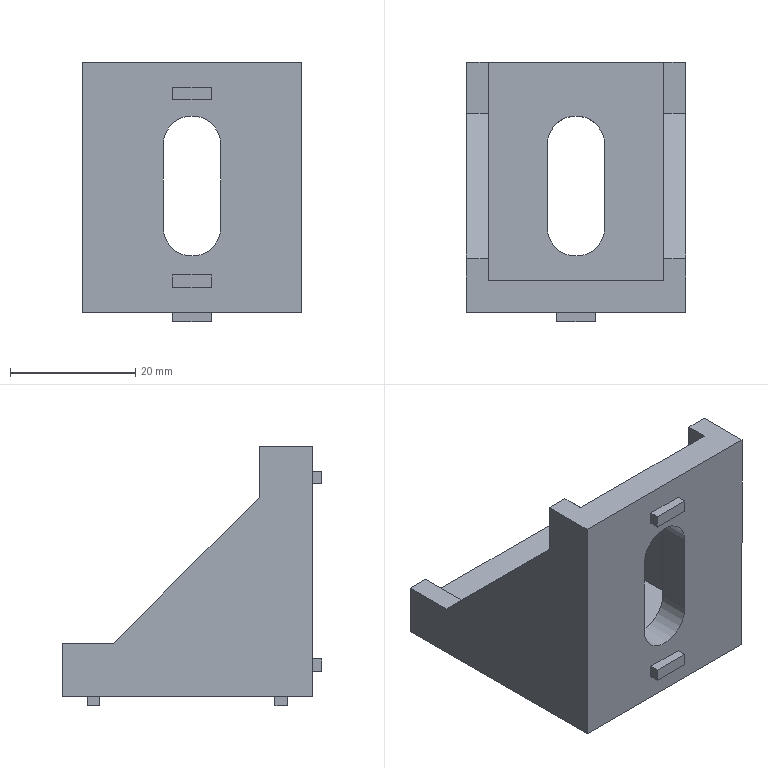Part | 1 solid | 44 faces | box 35 x 41.5 x 41.5 mm | volume 14850 mm3 | plane 40 | cylinder 4 | commonest cylinder face diameters 9.2 x4
STEP:
#1=CARTESIAN_POINT('',(14.,5.,5.));
#2=VERTEX_POINT('',#1);
#3=CARTESIAN_POINT('',(-14.,5.,5.));
#4=VERTEX_POINT('',#3);
#5=CARTESIAN_POINT('',(-17.5,5.,5.));
#6=DIRECTION('',(-1.,0.,0.));
#7=VECTOR('',#6,1000.);
#8=LINE('',#5,#7);
#9=EDGE_CURVE('',#2,#4,#8,.T.);
#10=ORIENTED_EDGE('',*,*,#9,.F.);
#11=CARTESIAN_POINT('',(14.,40.,5.));
#12=VERTEX_POINT('',#11);
#13=CARTESIAN_POINT('',(14.,0.,5.));
#14=DIRECTION('',(0.,-1.,0.));
#15=VECTOR('',#14,1000.);
#16=LINE('',#13,#15);
#17=EDGE_CURVE('',#12,#2,#16,.T.);
#18=ORIENTED_EDGE('',*,*,#17,.F.);
#19=CARTESIAN_POINT('',(-14.,40.,5.));
#20=VERTEX_POINT('',#19);
#21=CARTESIAN_POINT('',(-17.5,40.,5.));
#22=DIRECTION('',(-1.,0.,0.));
#23=VECTOR('',#22,1000.);
#24=LINE('',#21,#23);
#25=EDGE_CURVE('',#12,#20,#24,.T.);
#26=ORIENTED_EDGE('',*,*,#25,.T.);
#27=CARTESIAN_POINT('',(-14.,0.,5.));
#28=DIRECTION('',(0.,-1.,0.));
#29=VECTOR('',#28,1000.);
#30=LINE('',#27,#29);
#31=EDGE_CURVE('',#20,#4,#30,.T.);
#32=ORIENTED_EDGE('',*,*,#31,.T.);
#33=EDGE_LOOP('',(#10,#18,#26,#32));
#34=FACE_OUTER_BOUND('',#33,.T.);
#35=CARTESIAN_POINT('',(-4.6,26.8,5.));
#36=VERTEX_POINT('',#35);
#37=CARTESIAN_POINT('',(-4.6,13.6,5.));
#38=VERTEX_POINT('',#37);
#39=CARTESIAN_POINT('',(-4.6,26.8,5.));
#40=DIRECTION('',(0.,-1.,0.));
#41=VECTOR('',#40,1000.);
#42=LINE('',#39,#41);
#43=EDGE_CURVE('',#36,#38,#42,.T.);
#44=ORIENTED_EDGE('',*,*,#43,.F.);
#45=CARTESIAN_POINT('',(4.6,26.8,5.));
#46=VERTEX_POINT('',#45);
#47=CARTESIAN_POINT('',(0.,26.8,5.));
#48=DIRECTION('',(0.,0.,1.));
#49=DIRECTION('',(1.,0.,0.));
#50=AXIS2_PLACEMENT_3D('',#47,#48,#49);
#51=CIRCLE('',#50,4.6);
#52=EDGE_CURVE('',#46,#36,#51,.T.);
#53=ORIENTED_EDGE('',*,*,#52,.F.);
#54=CARTESIAN_POINT('',(4.6,13.6,5.));
#55=VERTEX_POINT('',#54);
#56=CARTESIAN_POINT('',(4.6,26.8,5.));
#57=DIRECTION('',(0.,1.,0.));
#58=VECTOR('',#57,1000.);
#59=LINE('',#56,#58);
#60=EDGE_CURVE('',#55,#46,#59,.T.);
#61=ORIENTED_EDGE('',*,*,#60,.F.);
#62=CARTESIAN_POINT('',(0.,13.6,5.));
#63=DIRECTION('',(0.,0.,1.));
#64=DIRECTION('',(1.,0.,0.));
#65=AXIS2_PLACEMENT_3D('',#62,#63,#64);
#66=CIRCLE('',#65,4.6);
#67=EDGE_CURVE('',#38,#55,#66,.T.);
#68=ORIENTED_EDGE('',*,*,#67,.F.);
#69=EDGE_LOOP('',(#44,#53,#61,#68));
#70=FACE_BOUND('',#69,.T.);
#71=CARTESIAN_POINT('',(-17.5,0.,5.));
#72=DIRECTION('',(0.,0.,1.));
#73=DIRECTION('',(1.,0.,0.));
#74=AXIS2_PLACEMENT_3D('',#71,#72,#73);
#75=PLANE('',#74);
#76=ADVANCED_FACE('',(#34,#70),#75,.T.);
#77=CARTESIAN_POINT('',(17.5,40.,0.));
#78=VERTEX_POINT('',#77);
#79=CARTESIAN_POINT('',(-17.5,40.,0.));
#80=VERTEX_POINT('',#79);
#81=CARTESIAN_POINT('',(-17.5,40.,0.));
#82=DIRECTION('',(-1.,0.,0.));
#83=VECTOR('',#82,1000.);
#84=LINE('',#81,#83);
#85=EDGE_CURVE('',#78,#80,#84,.T.);
#86=ORIENTED_EDGE('',*,*,#85,.F.);
#87=CARTESIAN_POINT('',(17.5,0.,0.));
#88=VERTEX_POINT('',#87);
#89=CARTESIAN_POINT('',(17.5,40.,0.));
#90=DIRECTION('',(0.,1.,0.));
#91=VECTOR('',#90,1000.);
#92=LINE('',#89,#91);
#93=EDGE_CURVE('',#88,#78,#92,.T.);
#94=ORIENTED_EDGE('',*,*,#93,.F.);
#95=CARTESIAN_POINT('',(-17.5,0.,0.));
#96=VERTEX_POINT('',#95);
#97=CARTESIAN_POINT('',(-17.5,0.,0.));
#98=DIRECTION('',(1.,0.,0.));
#99=VECTOR('',#98,1000.);
#100=LINE('',#97,#99);
#101=EDGE_CURVE('',#96,#88,#100,.T.);
#102=ORIENTED_EDGE('',*,*,#101,.F.);
#103=CARTESIAN_POINT('',(-17.5,40.,0.));
#104=DIRECTION('',(0.,-1.,0.));
#105=VECTOR('',#104,1000.);
#106=LINE('',#103,#105);
#107=EDGE_CURVE('',#80,#96,#106,.T.);
#108=ORIENTED_EDGE('',*,*,#107,.F.);
#109=EDGE_LOOP('',(#86,#94,#102,#108));
#110=FACE_OUTER_BOUND('',#109,.T.);
#111=CARTESIAN_POINT('',(3.1,34.,0.));
#112=VERTEX_POINT('',#111);
#113=CARTESIAN_POINT('',(-3.1,34.,0.));
#114=VERTEX_POINT('',#113);
#115=CARTESIAN_POINT('',(3.1,34.,0.));
#116=DIRECTION('',(-1.,0.,0.));
#117=VECTOR('',#116,1000.);
#118=LINE('',#115,#117);
#119=EDGE_CURVE('',#112,#114,#118,.T.);
#120=ORIENTED_EDGE('',*,*,#119,.F.);
#121=CARTESIAN_POINT('',(3.1,36.,0.));
#122=VERTEX_POINT('',#121);
#123=CARTESIAN_POINT('',(3.1,36.,0.));
#124=DIRECTION('',(0.,-1.,0.));
#125=VECTOR('',#124,1000.);
#126=LINE('',#123,#125);
#127=EDGE_CURVE('',#122,#112,#126,.T.);
#128=ORIENTED_EDGE('',*,*,#127,.F.);
#129=CARTESIAN_POINT('',(-3.1,36.,0.));
#130=VERTEX_POINT('',#129);
#131=CARTESIAN_POINT('',(3.1,36.,0.));
#132=DIRECTION('',(-1.,0.,0.));
#133=VECTOR('',#132,1000.);
#134=LINE('',#131,#133);
#135=EDGE_CURVE('',#122,#130,#134,.T.);
#136=ORIENTED_EDGE('',*,*,#135,.T.);
#137=CARTESIAN_POINT('',(-3.1,36.,0.));
#138=DIRECTION('',(0.,-1.,0.));
#139=VECTOR('',#138,1000.);
#140=LINE('',#137,#139);
#141=EDGE_CURVE('',#130,#114,#140,.T.);
#142=ORIENTED_EDGE('',*,*,#141,.T.);
#143=EDGE_LOOP('',(#120,#128,#136,#142));
#144=FACE_BOUND('',#143,.T.);
#145=CARTESIAN_POINT('',(3.1,4.,0.));
#146=VERTEX_POINT('',#145);
#147=CARTESIAN_POINT('',(-3.1,4.,0.));
#148=VERTEX_POINT('',#147);
#149=CARTESIAN_POINT('',(3.1,4.,0.));
#150=DIRECTION('',(-1.,0.,0.));
#151=VECTOR('',#150,1000.);
#152=LINE('',#149,#151);
#153=EDGE_CURVE('',#146,#148,#152,.T.);
#154=ORIENTED_EDGE('',*,*,#153,.F.);
#155=CARTESIAN_POINT('',(3.1,6.,0.));
#156=VERTEX_POINT('',#155);
#157=CARTESIAN_POINT('',(3.1,4.,0.));
#158=DIRECTION('',(0.,-1.,0.));
#159=VECTOR('',#158,1000.);
#160=LINE('',#157,#159);
#161=EDGE_CURVE('',#156,#146,#160,.T.);
#162=ORIENTED_EDGE('',*,*,#161,.F.);
#163=CARTESIAN_POINT('',(-3.1,6.,0.));
#164=VERTEX_POINT('',#163);
#165=CARTESIAN_POINT('',(3.1,6.,0.));
#166=DIRECTION('',(-1.,0.,0.));
#167=VECTOR('',#166,1000.);
#168=LINE('',#165,#167);
#169=EDGE_CURVE('',#156,#164,#168,.T.);
#170=ORIENTED_EDGE('',*,*,#169,.T.);
#171=CARTESIAN_POINT('',(-3.1,4.,0.));
#172=DIRECTION('',(0.,-1.,0.));
#173=VECTOR('',#172,1000.);
#174=LINE('',#171,#173);
#175=EDGE_CURVE('',#164,#148,#174,.T.);
#176=ORIENTED_EDGE('',*,*,#175,.T.);
#177=EDGE_LOOP('',(#154,#162,#170,#176));
#178=FACE_BOUND('',#177,.T.);
#179=CARTESIAN_POINT('',(4.6,26.8,0.));
#180=VERTEX_POINT('',#179);
#181=CARTESIAN_POINT('',(-4.6,26.8,0.));
#182=VERTEX_POINT('',#181);
#183=CARTESIAN_POINT('',(0.,26.8,0.));
#184=DIRECTION('',(0.,0.,1.));
#185=DIRECTION('',(1.,0.,0.));
#186=AXIS2_PLACEMENT_3D('',#183,#184,#185);
#187=CIRCLE('',#186,4.6);
#188=EDGE_CURVE('',#180,#182,#187,.T.);
#189=ORIENTED_EDGE('',*,*,#188,.T.);
#190=CARTESIAN_POINT('',(-4.6,13.6,0.));
#191=VERTEX_POINT('',#190);
#192=CARTESIAN_POINT('',(-4.6,26.8,0.));
#193=DIRECTION('',(0.,-1.,0.));
#194=VECTOR('',#193,1000.);
#195=LINE('',#192,#194);
#196=EDGE_CURVE('',#182,#191,#195,.T.);
#197=ORIENTED_EDGE('',*,*,#196,.T.);
#198=CARTESIAN_POINT('',(4.6,13.6,0.));
#199=VERTEX_POINT('',#198);
#200=CARTESIAN_POINT('',(0.,13.6,0.));
#201=DIRECTION('',(0.,0.,1.));
#202=DIRECTION('',(1.,0.,0.));
#203=AXIS2_PLACEMENT_3D('',#200,#201,#202);
#204=CIRCLE('',#203,4.6);
#205=EDGE_CURVE('',#191,#199,#204,.T.);
#206=ORIENTED_EDGE('',*,*,#205,.T.);
#207=CARTESIAN_POINT('',(4.6,26.8,0.));
#208=DIRECTION('',(0.,1.,0.));
#209=VECTOR('',#208,1000.);
#210=LINE('',#207,#209);
#211=EDGE_CURVE('',#199,#180,#210,.T.);
#212=ORIENTED_EDGE('',*,*,#211,.T.);
#213=EDGE_LOOP('',(#189,#197,#206,#212));
#214=FACE_BOUND('',#213,.T.);
#215=CARTESIAN_POINT('',(-17.5,0.,0.));
#216=DIRECTION('',(0.,0.,1.));
#217=DIRECTION('',(1.,0.,0.));
#218=AXIS2_PLACEMENT_3D('',#215,#216,#217);
#219=PLANE('',#218);
#220=ADVANCED_FACE('',(#110,#144,#178,#214),#219,.F.);
#221=ORIENTED_EDGE('',*,*,#107,.T.);
#222=CARTESIAN_POINT('',(-17.5,0.,40.));
#223=VERTEX_POINT('',#222);
#224=CARTESIAN_POINT('',(-17.5,0.,5.));
#225=DIRECTION('',(0.,0.,-1.));
#226=VECTOR('',#225,1000.);
#227=LINE('',#224,#226);
#228=EDGE_CURVE('',#223,#96,#227,.T.);
#229=ORIENTED_EDGE('',*,*,#228,.F.);
#230=CARTESIAN_POINT('',(-17.5,8.5,40.));
#231=VERTEX_POINT('',#230);
#232=CARTESIAN_POINT('',(-17.5,8.5,40.));
#233=DIRECTION('',(0.,1.,0.));
#234=VECTOR('',#233,1000.);
#235=LINE('',#232,#234);
#236=EDGE_CURVE('',#223,#231,#235,.T.);
#237=ORIENTED_EDGE('',*,*,#236,.T.);
#238=CARTESIAN_POINT('',(-17.5,8.5,31.8));
#239=VERTEX_POINT('',#238);
#240=CARTESIAN_POINT('',(-17.5,8.5,31.8));
#241=DIRECTION('',(0.,0.,-1.));
#242=VECTOR('',#241,1000.);
#243=LINE('',#240,#242);
#244=EDGE_CURVE('',#231,#239,#243,.T.);
#245=ORIENTED_EDGE('',*,*,#244,.T.);
#246=CARTESIAN_POINT('',(-17.5,31.8,8.5));
#247=VERTEX_POINT('',#246);
#248=CARTESIAN_POINT('',(-17.5,31.8,8.5));
#249=DIRECTION('',(0.,0.7071,-0.7071));
#250=VECTOR('',#249,1000.);
#251=LINE('',#248,#250);
#252=EDGE_CURVE('',#239,#247,#251,.T.);
#253=ORIENTED_EDGE('',*,*,#252,.T.);
#254=CARTESIAN_POINT('',(-17.5,40.,8.5));
#255=VERTEX_POINT('',#254);
#256=CARTESIAN_POINT('',(-17.5,40.,8.5));
#257=DIRECTION('',(0.,1.,0.));
#258=VECTOR('',#257,1000.);
#259=LINE('',#256,#258);
#260=EDGE_CURVE('',#247,#255,#259,.T.);
#261=ORIENTED_EDGE('',*,*,#260,.T.);
#262=CARTESIAN_POINT('',(-17.5,40.,5.));
#263=DIRECTION('',(0.,0.,-1.));
#264=VECTOR('',#263,1000.);
#265=LINE('',#262,#264);
#266=EDGE_CURVE('',#255,#80,#265,.T.);
#267=ORIENTED_EDGE('',*,*,#266,.T.);
#268=EDGE_LOOP('',(#221,#229,#237,#245,#253,#261,#267));
#269=FACE_OUTER_BOUND('',#268,.T.);
#270=CARTESIAN_POINT('',(-17.5,40.,5.));
#271=DIRECTION('',(1.,0.,0.));
#272=DIRECTION('',(0.,1.,0.));
#273=AXIS2_PLACEMENT_3D('',#270,#271,#272);
#274=PLANE('',#273);
#275=ADVANCED_FACE('',(#269),#274,.F.);
#276=CARTESIAN_POINT('',(17.5,0.,40.));
#277=VERTEX_POINT('',#276);
#278=CARTESIAN_POINT('',(17.5,0.,5.));
#279=DIRECTION('',(0.,0.,-1.));
#280=VECTOR('',#279,1000.);
#281=LINE('',#278,#280);
#282=EDGE_CURVE('',#277,#88,#281,.T.);
#283=ORIENTED_EDGE('',*,*,#282,.F.);
#284=CARTESIAN_POINT('',(-14.,0.,40.));
#285=DIRECTION('',(-1.,0.,0.));
#286=VECTOR('',#285,1000.);
#287=LINE('',#284,#286);
#288=EDGE_CURVE('',#277,#223,#287,.T.);
#289=ORIENTED_EDGE('',*,*,#288,.T.);
#290=ORIENTED_EDGE('',*,*,#228,.T.);
#291=ORIENTED_EDGE('',*,*,#101,.T.);
#292=EDGE_LOOP('',(#283,#289,#290,#291));
#293=FACE_OUTER_BOUND('',#292,.T.);
#294=CARTESIAN_POINT('',(3.1,0.,6.));
#295=VERTEX_POINT('',#294);
#296=CARTESIAN_POINT('',(-3.1,0.,6.));
#297=VERTEX_POINT('',#296);
#298=CARTESIAN_POINT('',(3.1,0.,6.));
#299=DIRECTION('',(-1.,0.,0.));
#300=VECTOR('',#299,1000.);
#301=LINE('',#298,#300);
#302=EDGE_CURVE('',#295,#297,#301,.T.);
#303=ORIENTED_EDGE('',*,*,#302,.F.);
#304=CARTESIAN_POINT('',(3.1,0.,4.));
#305=VERTEX_POINT('',#304);
#306=CARTESIAN_POINT('',(3.1,0.,4.));
#307=DIRECTION('',(0.,0.,1.));
#308=VECTOR('',#307,1000.);
#309=LINE('',#306,#308);
#310=EDGE_CURVE('',#305,#295,#309,.T.);
#311=ORIENTED_EDGE('',*,*,#310,.F.);
#312=CARTESIAN_POINT('',(-3.1,0.,4.));
#313=VERTEX_POINT('',#312);
#314=CARTESIAN_POINT('',(3.1,0.,4.));
#315=DIRECTION('',(-1.,0.,0.));
#316=VECTOR('',#315,1000.);
#317=LINE('',#314,#316);
#318=EDGE_CURVE('',#305,#313,#317,.T.);
#319=ORIENTED_EDGE('',*,*,#318,.T.);
#320=CARTESIAN_POINT('',(-3.1,0.,4.));
#321=DIRECTION('',(0.,0.,1.));
#322=VECTOR('',#321,1000.);
#323=LINE('',#320,#322);
#324=EDGE_CURVE('',#313,#297,#323,.T.);
#325=ORIENTED_EDGE('',*,*,#324,.T.);
#326=EDGE_LOOP('',(#303,#311,#319,#325));
#327=FACE_BOUND('',#326,.T.);
#328=CARTESIAN_POINT('',(3.1,0.,36.));
#329=VERTEX_POINT('',#328);
#330=CARTESIAN_POINT('',(-3.1,0.,36.));
#331=VERTEX_POINT('',#330);
#332=CARTESIAN_POINT('',(3.1,0.,36.));
#333=DIRECTION('',(-1.,0.,0.));
#334=VECTOR('',#333,1000.);
#335=LINE('',#332,#334);
#336=EDGE_CURVE('',#329,#331,#335,.T.);
#337=ORIENTED_EDGE('',*,*,#336,.F.);
#338=CARTESIAN_POINT('',(3.1,0.,34.));
#339=VERTEX_POINT('',#338);
#340=CARTESIAN_POINT('',(3.1,0.,36.));
#341=DIRECTION('',(0.,0.,1.));
#342=VECTOR('',#341,1000.);
#343=LINE('',#340,#342);
#344=EDGE_CURVE('',#339,#329,#343,.T.);
#345=ORIENTED_EDGE('',*,*,#344,.F.);
#346=CARTESIAN_POINT('',(-3.1,0.,34.));
#347=VERTEX_POINT('',#346);
#348=CARTESIAN_POINT('',(3.1,0.,34.));
#349=DIRECTION('',(-1.,0.,0.));
#350=VECTOR('',#349,1000.);
#351=LINE('',#348,#350);
#352=EDGE_CURVE('',#339,#347,#351,.T.);
#353=ORIENTED_EDGE('',*,*,#352,.T.);
#354=CARTESIAN_POINT('',(-3.1,0.,36.));
#355=DIRECTION('',(0.,0.,1.));
#356=VECTOR('',#355,1000.);
#357=LINE('',#354,#356);
#358=EDGE_CURVE('',#347,#331,#357,.T.);
#359=ORIENTED_EDGE('',*,*,#358,.T.);
#360=EDGE_LOOP('',(#337,#345,#353,#359));
#361=FACE_BOUND('',#360,.T.);
#362=CARTESIAN_POINT('',(-4.6,0.,26.8));
#363=VERTEX_POINT('',#362);
#364=CARTESIAN_POINT('',(-4.6,0.,13.6));
#365=VERTEX_POINT('',#364);
#366=CARTESIAN_POINT('',(-4.6,0.,26.8));
#367=DIRECTION('',(0.,0.,-1.));
#368=VECTOR('',#367,1000.);
#369=LINE('',#366,#368);
#370=EDGE_CURVE('',#363,#365,#369,.T.);
#371=ORIENTED_EDGE('',*,*,#370,.F.);
#372=CARTESIAN_POINT('',(4.6,0.,26.8));
#373=VERTEX_POINT('',#372);
#374=CARTESIAN_POINT('',(0.,0.,26.8));
#375=DIRECTION('',(0.,-1.,0.));
#376=DIRECTION('',(1.,0.,0.));
#377=AXIS2_PLACEMENT_3D('',#374,#375,#376);
#378=CIRCLE('',#377,4.6);
#379=EDGE_CURVE('',#373,#363,#378,.T.);
#380=ORIENTED_EDGE('',*,*,#379,.F.);
#381=CARTESIAN_POINT('',(4.6,0.,13.6));
#382=VERTEX_POINT('',#381);
#383=CARTESIAN_POINT('',(4.6,0.,26.8));
#384=DIRECTION('',(0.,0.,1.));
#385=VECTOR('',#384,1000.);
#386=LINE('',#383,#385);
#387=EDGE_CURVE('',#382,#373,#386,.T.);
#388=ORIENTED_EDGE('',*,*,#387,.F.);
#389=CARTESIAN_POINT('',(0.,0.,13.6));
#390=DIRECTION('',(0.,-1.,0.));
#391=DIRECTION('',(1.,0.,0.));
#392=AXIS2_PLACEMENT_3D('',#389,#390,#391);
#393=CIRCLE('',#392,4.6);
#394=EDGE_CURVE('',#365,#382,#393,.T.);
#395=ORIENTED_EDGE('',*,*,#394,.F.);
#396=EDGE_LOOP('',(#371,#380,#388,#395));
#397=FACE_BOUND('',#396,.T.);
#398=CARTESIAN_POINT('',(-17.5,0.,5.));
#399=DIRECTION('',(0.,1.,0.));
#400=DIRECTION('',(1.,0.,0.));
#401=AXIS2_PLACEMENT_3D('',#398,#399,#400);
#402=PLANE('',#401);
#403=ADVANCED_FACE('',(#293,#327,#361,#397),#402,.F.);
#404=CARTESIAN_POINT('',(17.5,8.5,40.));
#405=VERTEX_POINT('',#404);
#406=CARTESIAN_POINT('',(17.5,8.5,31.8));
#407=VERTEX_POINT('',#406);
#408=CARTESIAN_POINT('',(17.5,8.5,31.8));
#409=DIRECTION('',(0.,0.,-1.));
#410=VECTOR('',#409,1000.);
#411=LINE('',#408,#410);
#412=EDGE_CURVE('',#405,#407,#411,.T.);
#413=ORIENTED_EDGE('',*,*,#412,.F.);
#414=CARTESIAN_POINT('',(17.5,8.5,40.));
#415=DIRECTION('',(0.,1.,0.));
#416=VECTOR('',#415,1000.);
#417=LINE('',#414,#416);
#418=EDGE_CURVE('',#277,#405,#417,.T.);
#419=ORIENTED_EDGE('',*,*,#418,.F.);
#420=ORIENTED_EDGE('',*,*,#282,.T.);
#421=ORIENTED_EDGE('',*,*,#93,.T.);
#422=CARTESIAN_POINT('',(17.5,40.,8.5));
#423=VERTEX_POINT('',#422);
#424=CARTESIAN_POINT('',(17.5,40.,5.));
#425=DIRECTION('',(0.,0.,-1.));
#426=VECTOR('',#425,1000.);
#427=LINE('',#424,#426);
#428=EDGE_CURVE('',#423,#78,#427,.T.);
#429=ORIENTED_EDGE('',*,*,#428,.F.);
#430=CARTESIAN_POINT('',(17.5,31.8,8.5));
#431=VERTEX_POINT('',#430);
#432=CARTESIAN_POINT('',(17.5,40.,8.5));
#433=DIRECTION('',(0.,1.,0.));
#434=VECTOR('',#433,1000.);
#435=LINE('',#432,#434);
#436=EDGE_CURVE('',#431,#423,#435,.T.);
#437=ORIENTED_EDGE('',*,*,#436,.F.);
#438=CARTESIAN_POINT('',(17.5,31.8,8.5));
#439=DIRECTION('',(0.,0.7071,-0.7071));
#440=VECTOR('',#439,1000.);
#441=LINE('',#438,#440);
#442=EDGE_CURVE('',#407,#431,#441,.T.);
#443=ORIENTED_EDGE('',*,*,#442,.F.);
#444=EDGE_LOOP('',(#413,#419,#420,#421,#429,#437,#443));
#445=FACE_OUTER_BOUND('',#444,.T.);
#446=CARTESIAN_POINT('',(17.5,40.,5.));
#447=DIRECTION('',(-1.,0.,0.));
#448=DIRECTION('',(0.,1.,0.));
#449=AXIS2_PLACEMENT_3D('',#446,#447,#448);
#450=PLANE('',#449);
#451=ADVANCED_FACE('',(#445),#450,.F.);
#452=ORIENTED_EDGE('',*,*,#85,.T.);
#453=ORIENTED_EDGE('',*,*,#266,.F.);
#454=CARTESIAN_POINT('',(-14.,40.,8.5));
#455=VERTEX_POINT('',#454);
#456=CARTESIAN_POINT('',(-14.,40.,8.5));
#457=DIRECTION('',(-1.,0.,0.));
#458=VECTOR('',#457,1000.);
#459=LINE('',#456,#458);
#460=EDGE_CURVE('',#455,#255,#459,.T.);
#461=ORIENTED_EDGE('',*,*,#460,.F.);
#462=CARTESIAN_POINT('',(-14.,40.,5.));
#463=DIRECTION('',(0.,0.,-1.));
#464=VECTOR('',#463,1000.);
#465=LINE('',#462,#464);
#466=EDGE_CURVE('',#455,#20,#465,.T.);
#467=ORIENTED_EDGE('',*,*,#466,.T.);
#468=ORIENTED_EDGE('',*,*,#25,.F.);
#469=CARTESIAN_POINT('',(14.,40.,8.5));
#470=VERTEX_POINT('',#469);
#471=CARTESIAN_POINT('',(14.,40.,5.));
#472=DIRECTION('',(0.,0.,-1.));
#473=VECTOR('',#472,1000.);
#474=LINE('',#471,#473);
#475=EDGE_CURVE('',#470,#12,#474,.T.);
#476=ORIENTED_EDGE('',*,*,#475,.F.);
#477=CARTESIAN_POINT('',(14.,40.,8.5));
#478=DIRECTION('',(1.,0.,0.));
#479=VECTOR('',#478,1000.);
#480=LINE('',#477,#479);
#481=EDGE_CURVE('',#470,#423,#480,.T.);
#482=ORIENTED_EDGE('',*,*,#481,.T.);
#483=ORIENTED_EDGE('',*,*,#428,.T.);
#484=EDGE_LOOP('',(#452,#453,#461,#467,#468,#476,#482,#483));
#485=FACE_OUTER_BOUND('',#484,.T.);
#486=CARTESIAN_POINT('',(-17.5,40.,5.));
#487=DIRECTION('',(0.,-1.,0.));
#488=DIRECTION('',(0.,0.,-1.));
#489=AXIS2_PLACEMENT_3D('',#486,#487,#488);
#490=PLANE('',#489);
#491=ADVANCED_FACE('',(#485),#490,.F.);
#492=ORIENTED_EDGE('',*,*,#188,.F.);
#493=CARTESIAN_POINT('',(4.6,26.8,5.));
#494=DIRECTION('',(0.,0.,-1.));
#495=VECTOR('',#494,1000.);
#496=LINE('',#493,#495);
#497=EDGE_CURVE('',#46,#180,#496,.T.);
#498=ORIENTED_EDGE('',*,*,#497,.F.);
#499=ORIENTED_EDGE('',*,*,#52,.T.);
#500=CARTESIAN_POINT('',(-4.6,26.8,5.));
#501=DIRECTION('',(0.,0.,-1.));
#502=VECTOR('',#501,1000.);
#503=LINE('',#500,#502);
#504=EDGE_CURVE('',#36,#182,#503,.T.);
#505=ORIENTED_EDGE('',*,*,#504,.T.);
#506=EDGE_LOOP('',(#492,#498,#499,#505));
#507=FACE_OUTER_BOUND('',#506,.T.);
#508=CARTESIAN_POINT('',(0.,26.8,5.));
#509=DIRECTION('',(0.,0.,-1.));
#510=DIRECTION('',(-1.,0.,0.));
#511=AXIS2_PLACEMENT_3D('',#508,#509,#510);
#512=CYLINDRICAL_SURFACE('',#511,4.6);
#513=ADVANCED_FACE('',(#507),#512,.F.);
#514=ORIENTED_EDGE('',*,*,#196,.F.);
#515=ORIENTED_EDGE('',*,*,#504,.F.);
#516=ORIENTED_EDGE('',*,*,#43,.T.);
#517=CARTESIAN_POINT('',(-4.6,13.6,5.));
#518=DIRECTION('',(0.,0.,-1.));
#519=VECTOR('',#518,1000.);
#520=LINE('',#517,#519);
#521=EDGE_CURVE('',#38,#191,#520,.T.);
#522=ORIENTED_EDGE('',*,*,#521,.T.);
#523=EDGE_LOOP('',(#514,#515,#516,#522));
#524=FACE_OUTER_BOUND('',#523,.T.);
#525=CARTESIAN_POINT('',(-4.6,26.8,5.));
#526=DIRECTION('',(1.,0.,0.));
#527=DIRECTION('',(0.,1.,0.));
#528=AXIS2_PLACEMENT_3D('',#525,#526,#527);
#529=PLANE('',#528);
#530=ADVANCED_FACE('',(#524),#529,.T.);
#531=ORIENTED_EDGE('',*,*,#205,.F.);
#532=ORIENTED_EDGE('',*,*,#521,.F.);
#533=ORIENTED_EDGE('',*,*,#67,.T.);
#534=CARTESIAN_POINT('',(4.6,13.6,5.));
#535=DIRECTION('',(0.,0.,-1.));
#536=VECTOR('',#535,1000.);
#537=LINE('',#534,#536);
#538=EDGE_CURVE('',#55,#199,#537,.T.);
#539=ORIENTED_EDGE('',*,*,#538,.T.);
#540=EDGE_LOOP('',(#531,#532,#533,#539));
#541=FACE_OUTER_BOUND('',#540,.T.);
#542=CARTESIAN_POINT('',(0.,13.6,5.));
#543=DIRECTION('',(0.,0.,-1.));
#544=DIRECTION('',(-1.,0.,0.));
#545=AXIS2_PLACEMENT_3D('',#542,#543,#544);
#546=CYLINDRICAL_SURFACE('',#545,4.6);
#547=ADVANCED_FACE('',(#541),#546,.F.);
#548=ORIENTED_EDGE('',*,*,#211,.F.);
#549=ORIENTED_EDGE('',*,*,#538,.F.);
#550=ORIENTED_EDGE('',*,*,#60,.T.);
#551=ORIENTED_EDGE('',*,*,#497,.T.);
#552=EDGE_LOOP('',(#548,#549,#550,#551));
#553=FACE_OUTER_BOUND('',#552,.T.);
#554=CARTESIAN_POINT('',(4.6,26.8,5.));
#555=DIRECTION('',(-1.,0.,0.));
#556=DIRECTION('',(0.,1.,0.));
#557=AXIS2_PLACEMENT_3D('',#554,#555,#556);
#558=PLANE('',#557);
#559=ADVANCED_FACE('',(#553),#558,.T.);
#560=ORIENTED_EDGE('',*,*,#260,.F.);
#561=CARTESIAN_POINT('',(-14.,31.8,8.5));
#562=VERTEX_POINT('',#561);
#563=CARTESIAN_POINT('',(-14.,31.8,8.5));
#564=DIRECTION('',(-1.,0.,0.));
#565=VECTOR('',#564,1000.);
#566=LINE('',#563,#565);
#567=EDGE_CURVE('',#562,#247,#566,.T.);
#568=ORIENTED_EDGE('',*,*,#567,.F.);
#569=CARTESIAN_POINT('',(-14.,40.,8.5));
#570=DIRECTION('',(0.,1.,0.));
#571=VECTOR('',#570,1000.);
#572=LINE('',#569,#571);
#573=EDGE_CURVE('',#562,#455,#572,.T.);
#574=ORIENTED_EDGE('',*,*,#573,.T.);
#575=ORIENTED_EDGE('',*,*,#460,.T.);
#576=EDGE_LOOP('',(#560,#568,#574,#575));
#577=FACE_OUTER_BOUND('',#576,.T.);
#578=CARTESIAN_POINT('',(-14.,40.,8.5));
#579=DIRECTION('',(0.,0.,1.));
#580=DIRECTION('',(0.,-1.,0.));
#581=AXIS2_PLACEMENT_3D('',#578,#579,#580);
#582=PLANE('',#581);
#583=ADVANCED_FACE('',(#577),#582,.T.);
#584=ORIENTED_EDGE('',*,*,#252,.F.);
#585=CARTESIAN_POINT('',(-14.,8.5,31.8));
#586=VERTEX_POINT('',#585);
#587=CARTESIAN_POINT('',(-14.,8.5,31.8));
#588=DIRECTION('',(-1.,0.,0.));
#589=VECTOR('',#588,1000.);
#590=LINE('',#587,#589);
#591=EDGE_CURVE('',#586,#239,#590,.T.);
#592=ORIENTED_EDGE('',*,*,#591,.F.);
#593=CARTESIAN_POINT('',(-14.,31.8,8.5));
#594=DIRECTION('',(0.,0.7071,-0.7071));
#595=VECTOR('',#594,1000.);
#596=LINE('',#593,#595);
#597=EDGE_CURVE('',#586,#562,#596,.T.);
#598=ORIENTED_EDGE('',*,*,#597,.T.);
#599=ORIENTED_EDGE('',*,*,#567,.T.);
#600=EDGE_LOOP('',(#584,#592,#598,#599));
#601=FACE_OUTER_BOUND('',#600,.T.);
#602=CARTESIAN_POINT('',(-14.,31.8,8.5));
#603=DIRECTION('',(0.,0.7071,0.7071));
#604=DIRECTION('',(1.,0.,0.));
#605=AXIS2_PLACEMENT_3D('',#602,#603,#604);
#606=PLANE('',#605);
#607=ADVANCED_FACE('',(#601),#606,.T.);
#608=ORIENTED_EDGE('',*,*,#244,.F.);
#609=CARTESIAN_POINT('',(-14.,8.5,40.));
#610=VERTEX_POINT('',#609);
#611=CARTESIAN_POINT('',(-14.,8.5,40.));
#612=DIRECTION('',(-1.,0.,0.));
#613=VECTOR('',#612,1000.);
#614=LINE('',#611,#613);
#615=EDGE_CURVE('',#610,#231,#614,.T.);
#616=ORIENTED_EDGE('',*,*,#615,.F.);
#617=CARTESIAN_POINT('',(-14.,8.5,31.8));
#618=DIRECTION('',(0.,0.,-1.));
#619=VECTOR('',#618,1000.);
#620=LINE('',#617,#619);
#621=EDGE_CURVE('',#610,#586,#620,.T.);
#622=ORIENTED_EDGE('',*,*,#621,.T.);
#623=ORIENTED_EDGE('',*,*,#591,.T.);
#624=EDGE_LOOP('',(#608,#616,#622,#623));
#625=FACE_OUTER_BOUND('',#624,.T.);
#626=CARTESIAN_POINT('',(-14.,8.5,31.8));
#627=DIRECTION('',(0.,1.,0.));
#628=DIRECTION('',(0.,0.,-1.));
#629=AXIS2_PLACEMENT_3D('',#626,#627,#628);
#630=PLANE('',#629);
#631=ADVANCED_FACE('',(#625),#630,.T.);
#632=ORIENTED_EDGE('',*,*,#615,.T.);
#633=ORIENTED_EDGE('',*,*,#236,.F.);
#634=ORIENTED_EDGE('',*,*,#288,.F.);
#635=ORIENTED_EDGE('',*,*,#418,.T.);
#636=CARTESIAN_POINT('',(14.,8.5,40.));
#637=VERTEX_POINT('',#636);
#638=CARTESIAN_POINT('',(14.,8.5,40.));
#639=DIRECTION('',(1.,0.,0.));
#640=VECTOR('',#639,1000.);
#641=LINE('',#638,#640);
#642=EDGE_CURVE('',#637,#405,#641,.T.);
#643=ORIENTED_EDGE('',*,*,#642,.F.);
#644=CARTESIAN_POINT('',(14.,5.,40.));
#645=VERTEX_POINT('',#644);
#646=CARTESIAN_POINT('',(14.,8.5,40.));
#647=DIRECTION('',(0.,1.,0.));
#648=VECTOR('',#647,1000.);
#649=LINE('',#646,#648);
#650=EDGE_CURVE('',#645,#637,#649,.T.);
#651=ORIENTED_EDGE('',*,*,#650,.F.);
#652=CARTESIAN_POINT('',(-14.,5.,40.));
#653=VERTEX_POINT('',#652);
#654=CARTESIAN_POINT('',(-17.5,5.,40.));
#655=DIRECTION('',(-1.,0.,0.));
#656=VECTOR('',#655,1000.);
#657=LINE('',#654,#656);
#658=EDGE_CURVE('',#645,#653,#657,.T.);
#659=ORIENTED_EDGE('',*,*,#658,.T.);
#660=CARTESIAN_POINT('',(-14.,8.5,40.));
#661=DIRECTION('',(0.,1.,0.));
#662=VECTOR('',#661,1000.);
#663=LINE('',#660,#662);
#664=EDGE_CURVE('',#653,#610,#663,.T.);
#665=ORIENTED_EDGE('',*,*,#664,.T.);
#666=EDGE_LOOP('',(#632,#633,#634,#635,#643,#651,#659,#665));
#667=FACE_OUTER_BOUND('',#666,.T.);
#668=CARTESIAN_POINT('',(-14.,8.5,40.));
#669=DIRECTION('',(0.,0.,1.));
#670=DIRECTION('',(1.,0.,0.));
#671=AXIS2_PLACEMENT_3D('',#668,#669,#670);
#672=PLANE('',#671);
#673=ADVANCED_FACE('',(#667),#672,.T.);
#674=CARTESIAN_POINT('',(-14.,5.,5.));
#675=DIRECTION('',(0.,0.,1.));
#676=VECTOR('',#675,1000.);
#677=LINE('',#674,#676);
#678=EDGE_CURVE('',#4,#653,#677,.T.);
#679=ORIENTED_EDGE('',*,*,#678,.F.);
#680=ORIENTED_EDGE('',*,*,#31,.F.);
#681=ORIENTED_EDGE('',*,*,#466,.F.);
#682=ORIENTED_EDGE('',*,*,#573,.F.);
#683=ORIENTED_EDGE('',*,*,#597,.F.);
#684=ORIENTED_EDGE('',*,*,#621,.F.);
#685=ORIENTED_EDGE('',*,*,#664,.F.);
#686=EDGE_LOOP('',(#679,#680,#681,#682,#683,#684,#685));
#687=FACE_OUTER_BOUND('',#686,.T.);
#688=CARTESIAN_POINT('',(-14.,40.,5.));
#689=DIRECTION('',(1.,0.,0.));
#690=DIRECTION('',(0.,1.,0.));
#691=AXIS2_PLACEMENT_3D('',#688,#689,#690);
#692=PLANE('',#691);
#693=ADVANCED_FACE('',(#687),#692,.T.);
#694=ORIENTED_EDGE('',*,*,#412,.T.);
#695=CARTESIAN_POINT('',(14.,8.5,31.8));
#696=VERTEX_POINT('',#695);
#697=CARTESIAN_POINT('',(14.,8.5,31.8));
#698=DIRECTION('',(1.,0.,0.));
#699=VECTOR('',#698,1000.);
#700=LINE('',#697,#699);
#701=EDGE_CURVE('',#696,#407,#700,.T.);
#702=ORIENTED_EDGE('',*,*,#701,.F.);
#703=CARTESIAN_POINT('',(14.,8.5,31.8));
#704=DIRECTION('',(0.,0.,-1.));
#705=VECTOR('',#704,1000.);
#706=LINE('',#703,#705);
#707=EDGE_CURVE('',#637,#696,#706,.T.);
#708=ORIENTED_EDGE('',*,*,#707,.F.);
#709=ORIENTED_EDGE('',*,*,#642,.T.);
#710=EDGE_LOOP('',(#694,#702,#708,#709));
#711=FACE_OUTER_BOUND('',#710,.T.);
#712=CARTESIAN_POINT('',(14.,8.5,31.8));
#713=DIRECTION('',(0.,-1.,0.));
#714=DIRECTION('',(-1.,0.,0.));
#715=AXIS2_PLACEMENT_3D('',#712,#713,#714);
#716=PLANE('',#715);
#717=ADVANCED_FACE('',(#711),#716,.F.);
#718=ORIENTED_EDGE('',*,*,#442,.T.);
#719=CARTESIAN_POINT('',(14.,31.8,8.5));
#720=VERTEX_POINT('',#719);
#721=CARTESIAN_POINT('',(14.,31.8,8.5));
#722=DIRECTION('',(1.,0.,0.));
#723=VECTOR('',#722,1000.);
#724=LINE('',#721,#723);
#725=EDGE_CURVE('',#720,#431,#724,.T.);
#726=ORIENTED_EDGE('',*,*,#725,.F.);
#727=CARTESIAN_POINT('',(14.,31.8,8.5));
#728=DIRECTION('',(0.,0.7071,-0.7071));
#729=VECTOR('',#728,1000.);
#730=LINE('',#727,#729);
#731=EDGE_CURVE('',#696,#720,#730,.T.);
#732=ORIENTED_EDGE('',*,*,#731,.F.);
#733=ORIENTED_EDGE('',*,*,#701,.T.);
#734=EDGE_LOOP('',(#718,#726,#732,#733));
#735=FACE_OUTER_BOUND('',#734,.T.);
#736=CARTESIAN_POINT('',(14.,31.8,8.5));
#737=DIRECTION('',(0.,-0.7071,-0.7071));
#738=DIRECTION('',(0.,-0.7071,0.7071));
#739=AXIS2_PLACEMENT_3D('',#736,#737,#738);
#740=PLANE('',#739);
#741=ADVANCED_FACE('',(#735),#740,.F.);
#742=ORIENTED_EDGE('',*,*,#436,.T.);
#743=ORIENTED_EDGE('',*,*,#481,.F.);
#744=CARTESIAN_POINT('',(14.,40.,8.5));
#745=DIRECTION('',(0.,1.,0.));
#746=VECTOR('',#745,1000.);
#747=LINE('',#744,#746);
#748=EDGE_CURVE('',#720,#470,#747,.T.);
#749=ORIENTED_EDGE('',*,*,#748,.F.);
#750=ORIENTED_EDGE('',*,*,#725,.T.);
#751=EDGE_LOOP('',(#742,#743,#749,#750));
#752=FACE_OUTER_BOUND('',#751,.T.);
#753=CARTESIAN_POINT('',(14.,40.,8.5));
#754=DIRECTION('',(0.,0.,-1.));
#755=DIRECTION('',(0.,-1.,0.));
#756=AXIS2_PLACEMENT_3D('',#753,#754,#755);
#757=PLANE('',#756);
#758=ADVANCED_FACE('',(#752),#757,.F.);
#759=CARTESIAN_POINT('',(14.,5.,5.));
#760=DIRECTION('',(0.,0.,-1.));
#761=VECTOR('',#760,1000.);
#762=LINE('',#759,#761);
#763=EDGE_CURVE('',#645,#2,#762,.T.);
#764=ORIENTED_EDGE('',*,*,#763,.F.);
#765=ORIENTED_EDGE('',*,*,#650,.T.);
#766=ORIENTED_EDGE('',*,*,#707,.T.);
#767=ORIENTED_EDGE('',*,*,#731,.T.);
#768=ORIENTED_EDGE('',*,*,#748,.T.);
#769=ORIENTED_EDGE('',*,*,#475,.T.);
#770=ORIENTED_EDGE('',*,*,#17,.T.);
#771=EDGE_LOOP('',(#764,#765,#766,#767,#768,#769,#770));
#772=FACE_OUTER_BOUND('',#771,.T.);
#773=CARTESIAN_POINT('',(14.,40.,5.));
#774=DIRECTION('',(-1.,0.,0.));
#775=DIRECTION('',(0.,0.,1.));
#776=AXIS2_PLACEMENT_3D('',#773,#774,#775);
#777=PLANE('',#776);
#778=ADVANCED_FACE('',(#772),#777,.T.);
#779=ORIENTED_EDGE('',*,*,#9,.T.);
#780=ORIENTED_EDGE('',*,*,#678,.T.);
#781=ORIENTED_EDGE('',*,*,#658,.F.);
#782=ORIENTED_EDGE('',*,*,#763,.T.);
#783=EDGE_LOOP('',(#779,#780,#781,#782));
#784=FACE_OUTER_BOUND('',#783,.T.);
#785=CARTESIAN_POINT('',(4.6,5.,26.8));
#786=VERTEX_POINT('',#785);
#787=CARTESIAN_POINT('',(-4.6,5.,26.8));
#788=VERTEX_POINT('',#787);
#789=CARTESIAN_POINT('',(0.,5.,26.8));
#790=DIRECTION('',(0.,-1.,0.));
#791=DIRECTION('',(1.,0.,0.));
#792=AXIS2_PLACEMENT_3D('',#789,#790,#791);
#793=CIRCLE('',#792,4.6);
#794=EDGE_CURVE('',#786,#788,#793,.T.);
#795=ORIENTED_EDGE('',*,*,#794,.T.);
#796=CARTESIAN_POINT('',(-4.6,5.,13.6));
#797=VERTEX_POINT('',#796);
#798=CARTESIAN_POINT('',(-4.6,5.,26.8));
#799=DIRECTION('',(0.,0.,-1.));
#800=VECTOR('',#799,1000.);
#801=LINE('',#798,#800);
#802=EDGE_CURVE('',#788,#797,#801,.T.);
#803=ORIENTED_EDGE('',*,*,#802,.T.);
#804=CARTESIAN_POINT('',(4.6,5.,13.6));
#805=VERTEX_POINT('',#804);
#806=CARTESIAN_POINT('',(0.,5.,13.6));
#807=DIRECTION('',(0.,-1.,0.));
#808=DIRECTION('',(1.,0.,0.));
#809=AXIS2_PLACEMENT_3D('',#806,#807,#808);
#810=CIRCLE('',#809,4.6);
#811=EDGE_CURVE('',#797,#805,#810,.T.);
#812=ORIENTED_EDGE('',*,*,#811,.T.);
#813=CARTESIAN_POINT('',(4.6,5.,26.8));
#814=DIRECTION('',(0.,0.,1.));
#815=VECTOR('',#814,1000.);
#816=LINE('',#813,#815);
#817=EDGE_CURVE('',#805,#786,#816,.T.);
#818=ORIENTED_EDGE('',*,*,#817,.T.);
#819=EDGE_LOOP('',(#795,#803,#812,#818));
#820=FACE_BOUND('',#819,.T.);
#821=CARTESIAN_POINT('',(-17.5,5.,40.));
#822=DIRECTION('',(0.,1.,0.));
#823=DIRECTION('',(1.,0.,0.));
#824=AXIS2_PLACEMENT_3D('',#821,#822,#823);
#825=PLANE('',#824);
#826=ADVANCED_FACE('',(#784,#820),#825,.T.);
#827=ORIENTED_EDGE('',*,*,#379,.T.);
#828=CARTESIAN_POINT('',(-4.6,5.,26.8));
#829=DIRECTION('',(0.,-1.,0.));
#830=VECTOR('',#829,1000.);
#831=LINE('',#828,#830);
#832=EDGE_CURVE('',#788,#363,#831,.T.);
#833=ORIENTED_EDGE('',*,*,#832,.F.);
#834=ORIENTED_EDGE('',*,*,#794,.F.);
#835=CARTESIAN_POINT('',(4.6,5.,26.8));
#836=DIRECTION('',(0.,-1.,0.));
#837=VECTOR('',#836,1000.);
#838=LINE('',#835,#837);
#839=EDGE_CURVE('',#786,#373,#838,.T.);
#840=ORIENTED_EDGE('',*,*,#839,.T.);
#841=EDGE_LOOP('',(#827,#833,#834,#840));
#842=FACE_OUTER_BOUND('',#841,.T.);
#843=CARTESIAN_POINT('',(0.,5.,26.8));
#844=DIRECTION('',(0.,-1.,0.));
#845=DIRECTION('',(1.,0.,0.));
#846=AXIS2_PLACEMENT_3D('',#843,#844,#845);
#847=CYLINDRICAL_SURFACE('',#846,4.6);
#848=ADVANCED_FACE('',(#842),#847,.F.);
#849=ORIENTED_EDGE('',*,*,#387,.T.);
#850=ORIENTED_EDGE('',*,*,#839,.F.);
#851=ORIENTED_EDGE('',*,*,#817,.F.);
#852=CARTESIAN_POINT('',(4.6,5.,13.6));
#853=DIRECTION('',(0.,-1.,0.));
#854=VECTOR('',#853,1000.);
#855=LINE('',#852,#854);
#856=EDGE_CURVE('',#805,#382,#855,.T.);
#857=ORIENTED_EDGE('',*,*,#856,.T.);
#858=EDGE_LOOP('',(#849,#850,#851,#857));
#859=FACE_OUTER_BOUND('',#858,.T.);
#860=CARTESIAN_POINT('',(4.6,5.,26.8));
#861=DIRECTION('',(1.,0.,0.));
#862=DIRECTION('',(0.,1.,0.));
#863=AXIS2_PLACEMENT_3D('',#860,#861,#862);
#864=PLANE('',#863);
#865=ADVANCED_FACE('',(#859),#864,.F.);
#866=ORIENTED_EDGE('',*,*,#394,.T.);
#867=ORIENTED_EDGE('',*,*,#856,.F.);
#868=ORIENTED_EDGE('',*,*,#811,.F.);
#869=CARTESIAN_POINT('',(-4.6,5.,13.6));
#870=DIRECTION('',(0.,-1.,0.));
#871=VECTOR('',#870,1000.);
#872=LINE('',#869,#871);
#873=EDGE_CURVE('',#797,#365,#872,.T.);
#874=ORIENTED_EDGE('',*,*,#873,.T.);
#875=EDGE_LOOP('',(#866,#867,#868,#874));
#876=FACE_OUTER_BOUND('',#875,.T.);
#877=CARTESIAN_POINT('',(0.,5.,13.6));
#878=DIRECTION('',(0.,-1.,0.));
#879=DIRECTION('',(1.,0.,0.));
#880=AXIS2_PLACEMENT_3D('',#877,#878,#879);
#881=CYLINDRICAL_SURFACE('',#880,4.6);
#882=ADVANCED_FACE('',(#876),#881,.F.);
#883=ORIENTED_EDGE('',*,*,#370,.T.);
#884=ORIENTED_EDGE('',*,*,#873,.F.);
#885=ORIENTED_EDGE('',*,*,#802,.F.);
#886=ORIENTED_EDGE('',*,*,#832,.T.);
#887=EDGE_LOOP('',(#883,#884,#885,#886));
#888=FACE_OUTER_BOUND('',#887,.T.);
#889=CARTESIAN_POINT('',(-4.6,5.,26.8));
#890=DIRECTION('',(-1.,0.,0.));
#891=DIRECTION('',(0.,1.,0.));
#892=AXIS2_PLACEMENT_3D('',#889,#890,#891);
#893=PLANE('',#892);
#894=ADVANCED_FACE('',(#888),#893,.F.);
#895=CARTESIAN_POINT('',(-3.1,-1.5,36.));
#896=VERTEX_POINT('',#895);
#897=CARTESIAN_POINT('',(-3.1,0.,36.));
#898=DIRECTION('',(0.,-1.,0.));
#899=VECTOR('',#898,1000.);
#900=LINE('',#897,#899);
#901=EDGE_CURVE('',#331,#896,#900,.T.);
#902=ORIENTED_EDGE('',*,*,#901,.T.);
#903=CARTESIAN_POINT('',(3.1,-1.5,36.));
#904=VERTEX_POINT('',#903);
#905=CARTESIAN_POINT('',(3.1,-1.5,36.));
#906=DIRECTION('',(-1.,0.,0.));
#907=VECTOR('',#906,1000.);
#908=LINE('',#905,#907);
#909=EDGE_CURVE('',#904,#896,#908,.T.);
#910=ORIENTED_EDGE('',*,*,#909,.F.);
#911=CARTESIAN_POINT('',(3.1,0.,36.));
#912=DIRECTION('',(0.,-1.,0.));
#913=VECTOR('',#912,1000.);
#914=LINE('',#911,#913);
#915=EDGE_CURVE('',#329,#904,#914,.T.);
#916=ORIENTED_EDGE('',*,*,#915,.F.);
#917=ORIENTED_EDGE('',*,*,#336,.T.);
#918=EDGE_LOOP('',(#902,#910,#916,#917));
#919=FACE_OUTER_BOUND('',#918,.T.);
#920=CARTESIAN_POINT('',(3.1,0.,36.));
#921=DIRECTION('',(0.,0.,-1.));
#922=DIRECTION('',(0.,-1.,0.));
#923=AXIS2_PLACEMENT_3D('',#920,#921,#922);
#924=PLANE('',#923);
#925=ADVANCED_FACE('',(#919),#924,.F.);
#926=CARTESIAN_POINT('',(-3.1,-1.5,34.));
#927=VERTEX_POINT('',#926);
#928=CARTESIAN_POINT('',(-3.1,-1.5,36.));
#929=DIRECTION('',(0.,0.,-1.));
#930=VECTOR('',#929,1000.);
#931=LINE('',#928,#930);
#932=EDGE_CURVE('',#896,#927,#931,.T.);
#933=ORIENTED_EDGE('',*,*,#932,.T.);
#934=CARTESIAN_POINT('',(3.1,-1.5,34.));
#935=VERTEX_POINT('',#934);
#936=CARTESIAN_POINT('',(3.1,-1.5,34.));
#937=DIRECTION('',(-1.,0.,0.));
#938=VECTOR('',#937,1000.);
#939=LINE('',#936,#938);
#940=EDGE_CURVE('',#935,#927,#939,.T.);
#941=ORIENTED_EDGE('',*,*,#940,.F.);
#942=CARTESIAN_POINT('',(3.1,-1.5,36.));
#943=DIRECTION('',(0.,0.,-1.));
#944=VECTOR('',#943,1000.);
#945=LINE('',#942,#944);
#946=EDGE_CURVE('',#904,#935,#945,.T.);
#947=ORIENTED_EDGE('',*,*,#946,.F.);
#948=ORIENTED_EDGE('',*,*,#909,.T.);
#949=EDGE_LOOP('',(#933,#941,#947,#948));
#950=FACE_OUTER_BOUND('',#949,.T.);
#951=CARTESIAN_POINT('',(3.1,-1.5,36.));
#952=DIRECTION('',(0.,1.,0.));
#953=DIRECTION('',(0.,0.,-1.));
#954=AXIS2_PLACEMENT_3D('',#951,#952,#953);
#955=PLANE('',#954);
#956=ADVANCED_FACE('',(#950),#955,.F.);
#957=CARTESIAN_POINT('',(-3.1,0.,34.));
#958=DIRECTION('',(0.,1.,0.));
#959=VECTOR('',#958,1000.);
#960=LINE('',#957,#959);
#961=EDGE_CURVE('',#927,#347,#960,.T.);
#962=ORIENTED_EDGE('',*,*,#961,.T.);
#963=ORIENTED_EDGE('',*,*,#352,.F.);
#964=CARTESIAN_POINT('',(3.1,0.,34.));
#965=DIRECTION('',(0.,1.,0.));
#966=VECTOR('',#965,1000.);
#967=LINE('',#964,#966);
#968=EDGE_CURVE('',#935,#339,#967,.T.);
#969=ORIENTED_EDGE('',*,*,#968,.F.);
#970=ORIENTED_EDGE('',*,*,#940,.T.);
#971=EDGE_LOOP('',(#962,#963,#969,#970));
#972=FACE_OUTER_BOUND('',#971,.T.);
#973=CARTESIAN_POINT('',(3.1,0.,34.));
#974=DIRECTION('',(0.,0.,1.));
#975=DIRECTION('',(1.,0.,0.));
#976=AXIS2_PLACEMENT_3D('',#973,#974,#975);
#977=PLANE('',#976);
#978=ADVANCED_FACE('',(#972),#977,.F.);
#979=ORIENTED_EDGE('',*,*,#915,.T.);
#980=ORIENTED_EDGE('',*,*,#946,.T.);
#981=ORIENTED_EDGE('',*,*,#968,.T.);
#982=ORIENTED_EDGE('',*,*,#344,.T.);
#983=EDGE_LOOP('',(#979,#980,#981,#982));
#984=FACE_OUTER_BOUND('',#983,.T.);
#985=CARTESIAN_POINT('',(3.1,0.,0.));
#986=DIRECTION('',(1.,0.,0.));
#987=DIRECTION('',(0.,1.,0.));
#988=AXIS2_PLACEMENT_3D('',#985,#986,#987);
#989=PLANE('',#988);
#990=ADVANCED_FACE('',(#984),#989,.T.);
#991=ORIENTED_EDGE('',*,*,#901,.F.);
#992=ORIENTED_EDGE('',*,*,#358,.F.);
#993=ORIENTED_EDGE('',*,*,#961,.F.);
#994=ORIENTED_EDGE('',*,*,#932,.F.);
#995=EDGE_LOOP('',(#991,#992,#993,#994));
#996=FACE_OUTER_BOUND('',#995,.T.);
#997=CARTESIAN_POINT('',(-3.1,0.,0.));
#998=DIRECTION('',(1.,0.,0.));
#999=DIRECTION('',(0.,1.,0.));
#1000=AXIS2_PLACEMENT_3D('',#997,#998,#999);
#1001=PLANE('',#1000);
#1002=ADVANCED_FACE('',(#996),#1001,.F.);
#1003=CARTESIAN_POINT('',(-3.1,-1.5,6.));
#1004=VERTEX_POINT('',#1003);
#1005=CARTESIAN_POINT('',(-3.1,0.,6.));
#1006=DIRECTION('',(0.,-1.,0.));
#1007=VECTOR('',#1006,1000.);
#1008=LINE('',#1005,#1007);
#1009=EDGE_CURVE('',#297,#1004,#1008,.T.);
#1010=ORIENTED_EDGE('',*,*,#1009,.T.);
#1011=CARTESIAN_POINT('',(3.1,-1.5,6.));
#1012=VERTEX_POINT('',#1011);
#1013=CARTESIAN_POINT('',(3.1,-1.5,6.));
#1014=DIRECTION('',(-1.,0.,0.));
#1015=VECTOR('',#1014,1000.);
#1016=LINE('',#1013,#1015);
#1017=EDGE_CURVE('',#1012,#1004,#1016,.T.);
#1018=ORIENTED_EDGE('',*,*,#1017,.F.);
#1019=CARTESIAN_POINT('',(3.1,0.,6.));
#1020=DIRECTION('',(0.,-1.,0.));
#1021=VECTOR('',#1020,1000.);
#1022=LINE('',#1019,#1021);
#1023=EDGE_CURVE('',#295,#1012,#1022,.T.);
#1024=ORIENTED_EDGE('',*,*,#1023,.F.);
#1025=ORIENTED_EDGE('',*,*,#302,.T.);
#1026=EDGE_LOOP('',(#1010,#1018,#1024,#1025));
#1027=FACE_OUTER_BOUND('',#1026,.T.);
#1028=CARTESIAN_POINT('',(3.1,0.,6.));
#1029=DIRECTION('',(0.,0.,-1.));
#1030=DIRECTION('',(0.,-1.,0.));
#1031=AXIS2_PLACEMENT_3D('',#1028,#1029,#1030);
#1032=PLANE('',#1031);
#1033=ADVANCED_FACE('',(#1027),#1032,.F.);
#1034=CARTESIAN_POINT('',(-3.1,-1.5,4.));
#1035=VERTEX_POINT('',#1034);
#1036=CARTESIAN_POINT('',(-3.1,-1.5,4.));
#1037=DIRECTION('',(0.,0.,-1.));
#1038=VECTOR('',#1037,1000.);
#1039=LINE('',#1036,#1038);
#1040=EDGE_CURVE('',#1004,#1035,#1039,.T.);
#1041=ORIENTED_EDGE('',*,*,#1040,.T.);
#1042=CARTESIAN_POINT('',(3.1,-1.5,4.));
#1043=VERTEX_POINT('',#1042);
#1044=CARTESIAN_POINT('',(3.1,-1.5,4.));
#1045=DIRECTION('',(-1.,0.,0.));
#1046=VECTOR('',#1045,1000.);
#1047=LINE('',#1044,#1046);
#1048=EDGE_CURVE('',#1043,#1035,#1047,.T.);
#1049=ORIENTED_EDGE('',*,*,#1048,.F.);
#1050=CARTESIAN_POINT('',(3.1,-1.5,4.));
#1051=DIRECTION('',(0.,0.,-1.));
#1052=VECTOR('',#1051,1000.);
#1053=LINE('',#1050,#1052);
#1054=EDGE_CURVE('',#1012,#1043,#1053,.T.);
#1055=ORIENTED_EDGE('',*,*,#1054,.F.);
#1056=ORIENTED_EDGE('',*,*,#1017,.T.);
#1057=EDGE_LOOP('',(#1041,#1049,#1055,#1056));
#1058=FACE_OUTER_BOUND('',#1057,.T.);
#1059=CARTESIAN_POINT('',(3.1,-1.5,4.));
#1060=DIRECTION('',(0.,1.,0.));
#1061=DIRECTION('',(0.,0.,-1.));
#1062=AXIS2_PLACEMENT_3D('',#1059,#1060,#1061);
#1063=PLANE('',#1062);
#1064=ADVANCED_FACE('',(#1058),#1063,.F.);
#1065=CARTESIAN_POINT('',(-3.1,0.,4.));
#1066=DIRECTION('',(0.,1.,0.));
#1067=VECTOR('',#1066,1000.);
#1068=LINE('',#1065,#1067);
#1069=EDGE_CURVE('',#1035,#313,#1068,.T.);
#1070=ORIENTED_EDGE('',*,*,#1069,.T.);
#1071=ORIENTED_EDGE('',*,*,#318,.F.);
#1072=CARTESIAN_POINT('',(3.1,0.,4.));
#1073=DIRECTION('',(0.,1.,0.));
#1074=VECTOR('',#1073,1000.);
#1075=LINE('',#1072,#1074);
#1076=EDGE_CURVE('',#1043,#305,#1075,.T.);
#1077=ORIENTED_EDGE('',*,*,#1076,.F.);
#1078=ORIENTED_EDGE('',*,*,#1048,.T.);
#1079=EDGE_LOOP('',(#1070,#1071,#1077,#1078));
#1080=FACE_OUTER_BOUND('',#1079,.T.);
#1081=CARTESIAN_POINT('',(3.1,0.,4.));
#1082=DIRECTION('',(0.,0.,1.));
#1083=DIRECTION('',(1.,0.,0.));
#1084=AXIS2_PLACEMENT_3D('',#1081,#1082,#1083);
#1085=PLANE('',#1084);
#1086=ADVANCED_FACE('',(#1080),#1085,.F.);
#1087=ORIENTED_EDGE('',*,*,#310,.T.);
#1088=ORIENTED_EDGE('',*,*,#1023,.T.);
#1089=ORIENTED_EDGE('',*,*,#1054,.T.);
#1090=ORIENTED_EDGE('',*,*,#1076,.T.);
#1091=EDGE_LOOP('',(#1087,#1088,#1089,#1090));
#1092=FACE_OUTER_BOUND('',#1091,.T.);
#1093=CARTESIAN_POINT('',(3.1,0.,0.));
#1094=DIRECTION('',(1.,0.,0.));
#1095=DIRECTION('',(0.,1.,0.));
#1096=AXIS2_PLACEMENT_3D('',#1093,#1094,#1095);
#1097=PLANE('',#1096);
#1098=ADVANCED_FACE('',(#1092),#1097,.T.);
#1099=ORIENTED_EDGE('',*,*,#324,.F.);
#1100=ORIENTED_EDGE('',*,*,#1069,.F.);
#1101=ORIENTED_EDGE('',*,*,#1040,.F.);
#1102=ORIENTED_EDGE('',*,*,#1009,.F.);
#1103=EDGE_LOOP('',(#1099,#1100,#1101,#1102));
#1104=FACE_OUTER_BOUND('',#1103,.T.);
#1105=CARTESIAN_POINT('',(-3.1,0.,0.));
#1106=DIRECTION('',(1.,0.,0.));
#1107=DIRECTION('',(0.,1.,0.));
#1108=AXIS2_PLACEMENT_3D('',#1105,#1106,#1107);
#1109=PLANE('',#1108);
#1110=ADVANCED_FACE('',(#1104),#1109,.F.);
#1111=CARTESIAN_POINT('',(-3.1,4.,-1.5));
#1112=VERTEX_POINT('',#1111);
#1113=CARTESIAN_POINT('',(-3.1,4.,0.));
#1114=DIRECTION('',(0.,0.,-1.));
#1115=VECTOR('',#1114,1000.);
#1116=LINE('',#1113,#1115);
#1117=EDGE_CURVE('',#148,#1112,#1116,.T.);
#1118=ORIENTED_EDGE('',*,*,#1117,.T.);
#1119=CARTESIAN_POINT('',(3.1,4.,-1.5));
#1120=VERTEX_POINT('',#1119);
#1121=CARTESIAN_POINT('',(3.1,4.,-1.5));
#1122=DIRECTION('',(-1.,0.,0.));
#1123=VECTOR('',#1122,1000.);
#1124=LINE('',#1121,#1123);
#1125=EDGE_CURVE('',#1120,#1112,#1124,.T.);
#1126=ORIENTED_EDGE('',*,*,#1125,.F.);
#1127=CARTESIAN_POINT('',(3.1,4.,0.));
#1128=DIRECTION('',(0.,0.,-1.));
#1129=VECTOR('',#1128,1000.);
#1130=LINE('',#1127,#1129);
#1131=EDGE_CURVE('',#146,#1120,#1130,.T.);
#1132=ORIENTED_EDGE('',*,*,#1131,.F.);
#1133=ORIENTED_EDGE('',*,*,#153,.T.);
#1134=EDGE_LOOP('',(#1118,#1126,#1132,#1133));
#1135=FACE_OUTER_BOUND('',#1134,.T.);
#1136=CARTESIAN_POINT('',(3.1,4.,0.));
#1137=DIRECTION('',(0.,1.,0.));
#1138=DIRECTION('',(0.,0.,-1.));
#1139=AXIS2_PLACEMENT_3D('',#1136,#1137,#1138);
#1140=PLANE('',#1139);
#1141=ADVANCED_FACE('',(#1135),#1140,.F.);
#1142=CARTESIAN_POINT('',(-3.1,6.,-1.5));
#1143=VERTEX_POINT('',#1142);
#1144=CARTESIAN_POINT('',(-3.1,4.,-1.5));
#1145=DIRECTION('',(0.,1.,0.));
#1146=VECTOR('',#1145,1000.);
#1147=LINE('',#1144,#1146);
#1148=EDGE_CURVE('',#1112,#1143,#1147,.T.);
#1149=ORIENTED_EDGE('',*,*,#1148,.T.);
#1150=CARTESIAN_POINT('',(3.1,6.,-1.5));
#1151=VERTEX_POINT('',#1150);
#1152=CARTESIAN_POINT('',(3.1,6.,-1.5));
#1153=DIRECTION('',(-1.,0.,0.));
#1154=VECTOR('',#1153,1000.);
#1155=LINE('',#1152,#1154);
#1156=EDGE_CURVE('',#1151,#1143,#1155,.T.);
#1157=ORIENTED_EDGE('',*,*,#1156,.F.);
#1158=CARTESIAN_POINT('',(3.1,4.,-1.5));
#1159=DIRECTION('',(0.,1.,0.));
#1160=VECTOR('',#1159,1000.);
#1161=LINE('',#1158,#1160);
#1162=EDGE_CURVE('',#1120,#1151,#1161,.T.);
#1163=ORIENTED_EDGE('',*,*,#1162,.F.);
#1164=ORIENTED_EDGE('',*,*,#1125,.T.);
#1165=EDGE_LOOP('',(#1149,#1157,#1163,#1164));
#1166=FACE_OUTER_BOUND('',#1165,.T.);
#1167=CARTESIAN_POINT('',(3.1,4.,-1.5));
#1168=DIRECTION('',(0.,0.,1.));
#1169=DIRECTION('',(0.,-1.,0.));
#1170=AXIS2_PLACEMENT_3D('',#1167,#1168,#1169);
#1171=PLANE('',#1170);
#1172=ADVANCED_FACE('',(#1166),#1171,.F.);
#1173=CARTESIAN_POINT('',(-3.1,6.,0.));
#1174=DIRECTION('',(0.,0.,1.));
#1175=VECTOR('',#1174,1000.);
#1176=LINE('',#1173,#1175);
#1177=EDGE_CURVE('',#1143,#164,#1176,.T.);
#1178=ORIENTED_EDGE('',*,*,#1177,.T.);
#1179=ORIENTED_EDGE('',*,*,#169,.F.);
#1180=CARTESIAN_POINT('',(3.1,6.,0.));
#1181=DIRECTION('',(0.,0.,1.));
#1182=VECTOR('',#1181,1000.);
#1183=LINE('',#1180,#1182);
#1184=EDGE_CURVE('',#1151,#156,#1183,.T.);
#1185=ORIENTED_EDGE('',*,*,#1184,.F.);
#1186=ORIENTED_EDGE('',*,*,#1156,.T.);
#1187=EDGE_LOOP('',(#1178,#1179,#1185,#1186));
#1188=FACE_OUTER_BOUND('',#1187,.T.);
#1189=CARTESIAN_POINT('',(3.1,6.,0.));
#1190=DIRECTION('',(0.,-1.,0.));
#1191=DIRECTION('',(0.,0.,-1.));
#1192=AXIS2_PLACEMENT_3D('',#1189,#1190,#1191);
#1193=PLANE('',#1192);
#1194=ADVANCED_FACE('',(#1188),#1193,.F.);
#1195=ORIENTED_EDGE('',*,*,#1131,.T.);
#1196=ORIENTED_EDGE('',*,*,#1162,.T.);
#1197=ORIENTED_EDGE('',*,*,#1184,.T.);
#1198=ORIENTED_EDGE('',*,*,#161,.T.);
#1199=EDGE_LOOP('',(#1195,#1196,#1197,#1198));
#1200=FACE_OUTER_BOUND('',#1199,.T.);
#1201=CARTESIAN_POINT('',(3.1,0.,0.));
#1202=DIRECTION('',(1.,0.,0.));
#1203=DIRECTION('',(0.,1.,0.));
#1204=AXIS2_PLACEMENT_3D('',#1201,#1202,#1203);
#1205=PLANE('',#1204);
#1206=ADVANCED_FACE('',(#1200),#1205,.T.);
#1207=ORIENTED_EDGE('',*,*,#1117,.F.);
#1208=ORIENTED_EDGE('',*,*,#175,.F.);
#1209=ORIENTED_EDGE('',*,*,#1177,.F.);
#1210=ORIENTED_EDGE('',*,*,#1148,.F.);
#1211=EDGE_LOOP('',(#1207,#1208,#1209,#1210));
#1212=FACE_OUTER_BOUND('',#1211,.T.);
#1213=CARTESIAN_POINT('',(-3.1,0.,0.));
#1214=DIRECTION('',(1.,0.,0.));
#1215=DIRECTION('',(0.,1.,0.));
#1216=AXIS2_PLACEMENT_3D('',#1213,#1214,#1215);
#1217=PLANE('',#1216);
#1218=ADVANCED_FACE('',(#1212),#1217,.F.);
#1219=CARTESIAN_POINT('',(-3.1,34.,-1.5));
#1220=VERTEX_POINT('',#1219);
#1221=CARTESIAN_POINT('',(-3.1,34.,0.));
#1222=DIRECTION('',(0.,0.,-1.));
#1223=VECTOR('',#1222,1000.);
#1224=LINE('',#1221,#1223);
#1225=EDGE_CURVE('',#114,#1220,#1224,.T.);
#1226=ORIENTED_EDGE('',*,*,#1225,.T.);
#1227=CARTESIAN_POINT('',(3.1,34.,-1.5));
#1228=VERTEX_POINT('',#1227);
#1229=CARTESIAN_POINT('',(3.1,34.,-1.5));
#1230=DIRECTION('',(-1.,0.,0.));
#1231=VECTOR('',#1230,1000.);
#1232=LINE('',#1229,#1231);
#1233=EDGE_CURVE('',#1228,#1220,#1232,.T.);
#1234=ORIENTED_EDGE('',*,*,#1233,.F.);
#1235=CARTESIAN_POINT('',(3.1,34.,0.));
#1236=DIRECTION('',(0.,0.,-1.));
#1237=VECTOR('',#1236,1000.);
#1238=LINE('',#1235,#1237);
#1239=EDGE_CURVE('',#112,#1228,#1238,.T.);
#1240=ORIENTED_EDGE('',*,*,#1239,.F.);
#1241=ORIENTED_EDGE('',*,*,#119,.T.);
#1242=EDGE_LOOP('',(#1226,#1234,#1240,#1241));
#1243=FACE_OUTER_BOUND('',#1242,.T.);
#1244=CARTESIAN_POINT('',(3.1,34.,0.));
#1245=DIRECTION('',(0.,1.,0.));
#1246=DIRECTION('',(0.,0.,-1.));
#1247=AXIS2_PLACEMENT_3D('',#1244,#1245,#1246);
#1248=PLANE('',#1247);
#1249=ADVANCED_FACE('',(#1243),#1248,.F.);
#1250=CARTESIAN_POINT('',(-3.1,36.,-1.5));
#1251=VERTEX_POINT('',#1250);
#1252=CARTESIAN_POINT('',(-3.1,36.,-1.5));
#1253=DIRECTION('',(0.,1.,0.));
#1254=VECTOR('',#1253,1000.);
#1255=LINE('',#1252,#1254);
#1256=EDGE_CURVE('',#1220,#1251,#1255,.T.);
#1257=ORIENTED_EDGE('',*,*,#1256,.T.);
#1258=CARTESIAN_POINT('',(3.1,36.,-1.5));
#1259=VERTEX_POINT('',#1258);
#1260=CARTESIAN_POINT('',(3.1,36.,-1.5));
#1261=DIRECTION('',(-1.,0.,0.));
#1262=VECTOR('',#1261,1000.);
#1263=LINE('',#1260,#1262);
#1264=EDGE_CURVE('',#1259,#1251,#1263,.T.);
#1265=ORIENTED_EDGE('',*,*,#1264,.F.);
#1266=CARTESIAN_POINT('',(3.1,36.,-1.5));
#1267=DIRECTION('',(0.,1.,0.));
#1268=VECTOR('',#1267,1000.);
#1269=LINE('',#1266,#1268);
#1270=EDGE_CURVE('',#1228,#1259,#1269,.T.);
#1271=ORIENTED_EDGE('',*,*,#1270,.F.);
#1272=ORIENTED_EDGE('',*,*,#1233,.T.);
#1273=EDGE_LOOP('',(#1257,#1265,#1271,#1272));
#1274=FACE_OUTER_BOUND('',#1273,.T.);
#1275=CARTESIAN_POINT('',(3.1,36.,-1.5));
#1276=DIRECTION('',(0.,0.,1.));
#1277=DIRECTION('',(0.,-1.,0.));
#1278=AXIS2_PLACEMENT_3D('',#1275,#1276,#1277);
#1279=PLANE('',#1278);
#1280=ADVANCED_FACE('',(#1274),#1279,.F.);
#1281=CARTESIAN_POINT('',(-3.1,36.,0.));
#1282=DIRECTION('',(0.,0.,1.));
#1283=VECTOR('',#1282,1000.);
#1284=LINE('',#1281,#1283);
#1285=EDGE_CURVE('',#1251,#130,#1284,.T.);
#1286=ORIENTED_EDGE('',*,*,#1285,.T.);
#1287=ORIENTED_EDGE('',*,*,#135,.F.);
#1288=CARTESIAN_POINT('',(3.1,36.,0.));
#1289=DIRECTION('',(0.,0.,1.));
#1290=VECTOR('',#1289,1000.);
#1291=LINE('',#1288,#1290);
#1292=EDGE_CURVE('',#1259,#122,#1291,.T.);
#1293=ORIENTED_EDGE('',*,*,#1292,.F.);
#1294=ORIENTED_EDGE('',*,*,#1264,.T.);
#1295=EDGE_LOOP('',(#1286,#1287,#1293,#1294));
#1296=FACE_OUTER_BOUND('',#1295,.T.);
#1297=CARTESIAN_POINT('',(3.1,36.,0.));
#1298=DIRECTION('',(0.,-1.,0.));
#1299=DIRECTION('',(0.,0.,-1.));
#1300=AXIS2_PLACEMENT_3D('',#1297,#1298,#1299);
#1301=PLANE('',#1300);
#1302=ADVANCED_FACE('',(#1296),#1301,.F.);
#1303=ORIENTED_EDGE('',*,*,#127,.T.);
#1304=ORIENTED_EDGE('',*,*,#1239,.T.);
#1305=ORIENTED_EDGE('',*,*,#1270,.T.);
#1306=ORIENTED_EDGE('',*,*,#1292,.T.);
#1307=EDGE_LOOP('',(#1303,#1304,#1305,#1306));
#1308=FACE_OUTER_BOUND('',#1307,.T.);
#1309=CARTESIAN_POINT('',(3.1,0.,0.));
#1310=DIRECTION('',(1.,0.,0.));
#1311=DIRECTION('',(0.,1.,0.));
#1312=AXIS2_PLACEMENT_3D('',#1309,#1310,#1311);
#1313=PLANE('',#1312);
#1314=ADVANCED_FACE('',(#1308),#1313,.T.);
#1315=ORIENTED_EDGE('',*,*,#141,.F.);
#1316=ORIENTED_EDGE('',*,*,#1285,.F.);
#1317=ORIENTED_EDGE('',*,*,#1256,.F.);
#1318=ORIENTED_EDGE('',*,*,#1225,.F.);
#1319=EDGE_LOOP('',(#1315,#1316,#1317,#1318));
#1320=FACE_OUTER_BOUND('',#1319,.T.);
#1321=CARTESIAN_POINT('',(-3.1,0.,0.));
#1322=DIRECTION('',(1.,0.,0.));
#1323=DIRECTION('',(0.,1.,0.));
#1324=AXIS2_PLACEMENT_3D('',#1321,#1322,#1323);
#1325=PLANE('',#1324);
#1326=ADVANCED_FACE('',(#1320),#1325,.F.);
#1327=CLOSED_SHELL('',(#76,#220,#275,#403,#451,#491,#513,#530,#547,#559,#583,#607,#631,#673,#693,#717,#741,#758,#778,#826,#848,#865,#882,#894,#925,#956,#978,#990,#1002,#1033,#1064,#1086,#1098,#1110,#1141,#1172,#1194,#1206,#1218,#1249,#1280,#1302,#1314,#1326));
#1328=MANIFOLD_SOLID_BREP('',#1327);
#1329=CARTESIAN_POINT('',(0.,0.,0.));
#1330=DIRECTION('',(0.,0.,1.));
#1331=DIRECTION('',(1.,0.,0.));
#1332=AXIS2_PLACEMENT_3D('',#1329,#1330,#1331);
#1333=(LENGTH_UNIT()NAMED_UNIT(*)SI_UNIT(.MILLI.,.METRE.));
#1334=UNCERTAINTY_MEASURE_WITH_UNIT(LENGTH_MEASURE(0.00001),#1333,'','');
#1335=(NAMED_UNIT(*)PLANE_ANGLE_UNIT()SI_UNIT($,.RADIAN.));
#1336=(NAMED_UNIT(*)SI_UNIT($,.STERADIAN.)SOLID_ANGLE_UNIT());
#1337=(GEOMETRIC_REPRESENTATION_CONTEXT(3)GLOBAL_UNCERTAINTY_ASSIGNED_CONTEXT((#1334))GLOBAL_UNIT_ASSIGNED_CONTEXT((#1333,#1335,#1336))REPRESENTATION_CONTEXT('',''));
#1338=ADVANCED_BREP_SHAPE_REPRESENTATION('',(#1328,#1332),#1337);